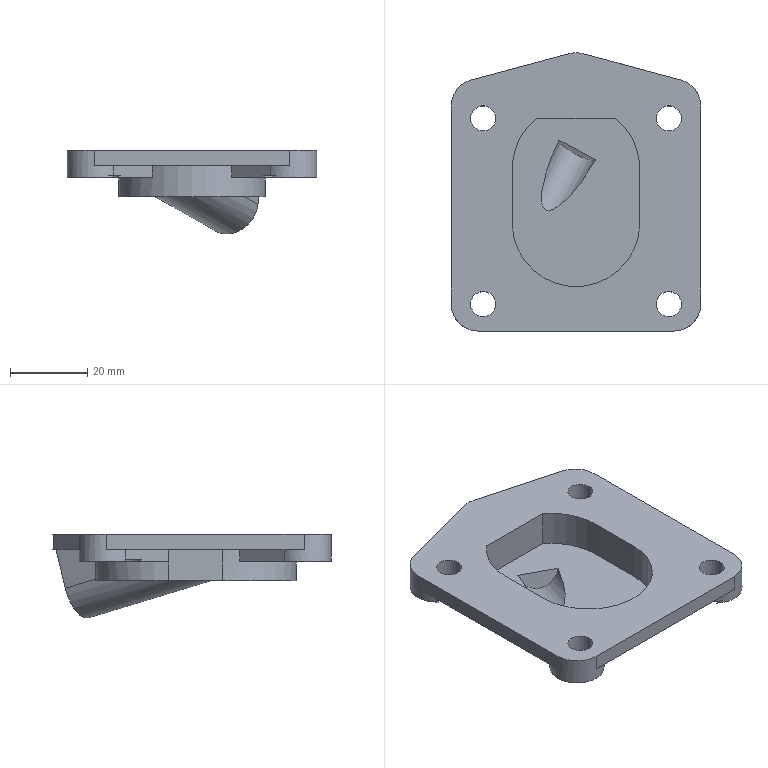Part | SolidWorks | features BaseBody 1 | 1 solid | 73 faces | box 64.5 x 72 x 21.727 mm | volume 23668 mm3 | plane 38 | cylinder 35 | commonest cylinder face diameters 12.5 x12 6.5 x8 14 x6 33 x3 38 x3 11 x1